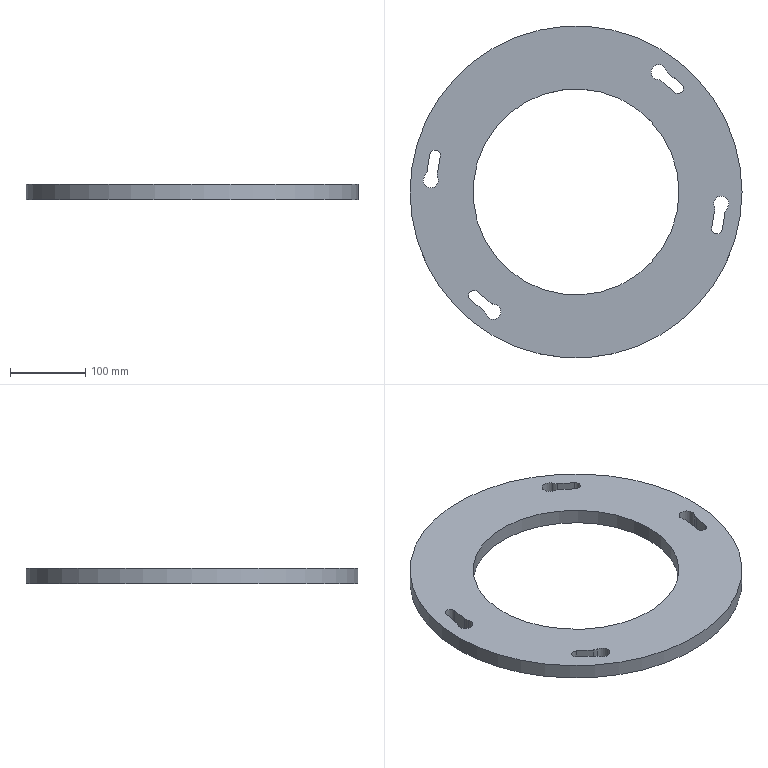Part | NX | 1 solid | 28 faces | box 440 x 440 x 20 mm | volume 1811359 mm3 | cylinder 18 | plane 10 | commonest cylinder face diameters 26 x8 14 x4 20 x4 273 x1 440 x1
STEP:
#1=CARTESIAN_POINT('',(182.981,-18.897,-20.));
#2=VERTEX_POINT('',#1);
#3=CARTESIAN_POINT('',(200.129,-21.798,-20.));
#4=VERTEX_POINT('',#3);
#5=CARTESIAN_POINT('',(192.378,-15.478,-20.));
#6=DIRECTION('',(0.,0.,-1.));
#7=DIRECTION('',(-1.,0.,0.));
#8=AXIS2_PLACEMENT_3D('',#5,#6,#7);
#9=CIRCLE('',#8,10.);
#10=EDGE_CURVE('',#2,#4,#9,.T.);
#11=ORIENTED_EDGE('',*,*,#10,.T.);
#12=CARTESIAN_POINT('',(200.129,-21.798,0.));
#13=VERTEX_POINT('',#12);
#14=CARTESIAN_POINT('',(200.129,-21.798,-20.));
#15=DIRECTION('',(0.,0.,1.));
#16=VECTOR('',#15,1000.);
#17=LINE('',#14,#16);
#18=EDGE_CURVE('',#4,#13,#17,.T.);
#19=ORIENTED_EDGE('',*,*,#18,.T.);
#20=CARTESIAN_POINT('',(182.981,-18.897,0.));
#21=VERTEX_POINT('',#20);
#22=CARTESIAN_POINT('',(192.378,-15.478,0.));
#23=DIRECTION('',(0.,0.,-1.));
#24=DIRECTION('',(-1.,0.,0.));
#25=AXIS2_PLACEMENT_3D('',#22,#23,#24);
#26=CIRCLE('',#25,10.);
#27=EDGE_CURVE('',#21,#13,#26,.T.);
#28=ORIENTED_EDGE('',*,*,#27,.F.);
#29=CARTESIAN_POINT('',(182.981,-18.897,-20.));
#30=DIRECTION('',(0.,0.,1.));
#31=VECTOR('',#30,1000.);
#32=LINE('',#29,#31);
#33=EDGE_CURVE('',#21,#2,#32,.F.);
#34=ORIENTED_EDGE('',*,*,#33,.T.);
#35=EDGE_LOOP('',(#11,#19,#28,#34));
#36=FACE_BOUND('',#35,.T.);
#37=CARTESIAN_POINT('',(192.378,-15.478,-20.));
#38=DIRECTION('',(0.,0.,1.));
#39=DIRECTION('',(1.,0.,0.));
#40=AXIS2_PLACEMENT_3D('',#37,#38,#39);
#41=CYLINDRICAL_SURFACE('',#40,10.);
#42=ADVANCED_FACE('',(#36),#41,.F.);
#43=CARTESIAN_POINT('',(197.386,-27.845,0.));
#44=VERTEX_POINT('',#43);
#45=CARTESIAN_POINT('',(193.67,-49.817,0.));
#46=VERTEX_POINT('',#45);
#47=CARTESIAN_POINT('',(198.089,-23.687,0.));
#48=DIRECTION('',(-0.1668,-0.986,0.));
#49=VECTOR('',#48,1000.);
#50=LINE('',#47,#49);
#51=EDGE_CURVE('',#44,#46,#50,.T.);
#52=ORIENTED_EDGE('',*,*,#51,.F.);
#53=CARTESIAN_POINT('',(197.386,-27.845,-20.));
#54=VERTEX_POINT('',#53);
#55=CARTESIAN_POINT('',(197.386,-27.845,-20.));
#56=DIRECTION('',(0.,0.,1.));
#57=VECTOR('',#56,1000.);
#58=LINE('',#55,#57);
#59=EDGE_CURVE('',#44,#54,#58,.F.);
#60=ORIENTED_EDGE('',*,*,#59,.T.);
#61=CARTESIAN_POINT('',(193.67,-49.817,-20.));
#62=VERTEX_POINT('',#61);
#63=CARTESIAN_POINT('',(198.089,-23.687,-20.));
#64=DIRECTION('',(-0.1668,-0.986,0.));
#65=VECTOR('',#64,1000.);
#66=LINE('',#63,#65);
#67=EDGE_CURVE('',#54,#62,#66,.T.);
#68=ORIENTED_EDGE('',*,*,#67,.T.);
#69=CARTESIAN_POINT('',(193.67,-49.817,-20.));
#70=DIRECTION('',(0.,0.,1.));
#71=VECTOR('',#70,1000.);
#72=LINE('',#69,#71);
#73=EDGE_CURVE('',#62,#46,#72,.T.);
#74=ORIENTED_EDGE('',*,*,#73,.T.);
#75=EDGE_LOOP('',(#52,#60,#68,#74));
#76=FACE_BOUND('',#75,.T.);
#77=CARTESIAN_POINT('',(198.089,-23.687,-20.));
#78=DIRECTION('',(-0.986,0.1668,0.));
#79=DIRECTION('',(-0.1668,-0.986,0.));
#80=AXIS2_PLACEMENT_3D('',#77,#78,#79);
#81=PLANE('',#80);
#82=ADVANCED_FACE('',(#76),#81,.T.);
#83=CARTESIAN_POINT('',(179.866,-47.482,0.));
#84=VERTEX_POINT('',#83);
#85=CARTESIAN_POINT('',(186.768,-48.649,0.));
#86=DIRECTION('',(0.,0.,-1.));
#87=DIRECTION('',(-1.,0.,0.));
#88=AXIS2_PLACEMENT_3D('',#85,#86,#87);
#89=CIRCLE('',#88,7.);
#90=EDGE_CURVE('',#46,#84,#89,.T.);
#91=ORIENTED_EDGE('',*,*,#90,.F.);
#92=ORIENTED_EDGE('',*,*,#73,.F.);
#93=CARTESIAN_POINT('',(179.866,-47.482,-20.));
#94=VERTEX_POINT('',#93);
#95=CARTESIAN_POINT('',(186.768,-48.649,-20.));
#96=DIRECTION('',(0.,0.,-1.));
#97=DIRECTION('',(-1.,0.,0.));
#98=AXIS2_PLACEMENT_3D('',#95,#96,#97);
#99=CIRCLE('',#98,7.);
#100=EDGE_CURVE('',#62,#94,#99,.T.);
#101=ORIENTED_EDGE('',*,*,#100,.T.);
#102=CARTESIAN_POINT('',(179.866,-47.482,-20.));
#103=DIRECTION('',(0.,0.,1.));
#104=VECTOR('',#103,1000.);
#105=LINE('',#102,#104);
#106=EDGE_CURVE('',#94,#84,#105,.T.);
#107=ORIENTED_EDGE('',*,*,#106,.T.);
#108=EDGE_LOOP('',(#91,#92,#101,#107));
#109=FACE_BOUND('',#108,.T.);
#110=CARTESIAN_POINT('',(186.768,-48.649,-20.));
#111=DIRECTION('',(0.,0.,1.));
#112=DIRECTION('',(1.,0.,0.));
#113=AXIS2_PLACEMENT_3D('',#110,#111,#112);
#114=CYLINDRICAL_SURFACE('',#113,7.);
#115=ADVANCED_FACE('',(#109),#114,.F.);
#116=CARTESIAN_POINT('',(139.978,142.815,0.));
#117=VERTEX_POINT('',#116);
#118=CARTESIAN_POINT('',(131.054,132.027,0.));
#119=VERTEX_POINT('',#118);
#120=CARTESIAN_POINT('',(135.516,137.421,0.));
#121=DIRECTION('',(0.,0.,-1.));
#122=DIRECTION('',(-1.,0.,0.));
#123=AXIS2_PLACEMENT_3D('',#120,#121,#122);
#124=CIRCLE('',#123,7.);
#125=EDGE_CURVE('',#117,#119,#124,.T.);
#126=ORIENTED_EDGE('',*,*,#125,.F.);
#127=CARTESIAN_POINT('',(139.978,142.815,-20.));
#128=VERTEX_POINT('',#127);
#129=CARTESIAN_POINT('',(139.978,142.815,-20.));
#130=DIRECTION('',(0.,0.,1.));
#131=VECTOR('',#130,1000.);
#132=LINE('',#129,#131);
#133=EDGE_CURVE('',#128,#117,#132,.T.);
#134=ORIENTED_EDGE('',*,*,#133,.F.);
#135=CARTESIAN_POINT('',(131.054,132.027,-20.));
#136=VERTEX_POINT('',#135);
#137=CARTESIAN_POINT('',(135.516,137.421,-20.));
#138=DIRECTION('',(0.,0.,-1.));
#139=DIRECTION('',(-1.,0.,0.));
#140=AXIS2_PLACEMENT_3D('',#137,#138,#139);
#141=CIRCLE('',#140,7.);
#142=EDGE_CURVE('',#128,#136,#141,.T.);
#143=ORIENTED_EDGE('',*,*,#142,.T.);
#144=CARTESIAN_POINT('',(131.054,132.027,-20.));
#145=DIRECTION('',(0.,0.,1.));
#146=VECTOR('',#145,1000.);
#147=LINE('',#144,#146);
#148=EDGE_CURVE('',#136,#119,#147,.T.);
#149=ORIENTED_EDGE('',*,*,#148,.T.);
#150=EDGE_LOOP('',(#126,#134,#143,#149));
#151=FACE_BOUND('',#150,.T.);
#152=CARTESIAN_POINT('',(135.516,137.421,-20.));
#153=DIRECTION('',(0.,0.,1.));
#154=DIRECTION('',(1.,0.,0.));
#155=AXIS2_PLACEMENT_3D('',#152,#153,#154);
#156=CYLINDRICAL_SURFACE('',#155,7.);
#157=ADVANCED_FACE('',(#151),#156,.F.);
#158=CARTESIAN_POINT('',(113.883,146.232,-20.));
#159=VERTEX_POINT('',#158);
#160=CARTESIAN_POINT('',(131.054,132.027,-20.));
#161=DIRECTION('',(-0.7705,0.6374,0.));
#162=VECTOR('',#161,1000.);
#163=LINE('',#160,#162);
#164=EDGE_CURVE('',#136,#159,#163,.T.);
#165=ORIENTED_EDGE('',*,*,#164,.T.);
#166=CARTESIAN_POINT('',(113.883,146.232,0.));
#167=VERTEX_POINT('',#166);
#168=CARTESIAN_POINT('',(113.883,146.232,-20.));
#169=DIRECTION('',(0.,0.,1.));
#170=VECTOR('',#169,1000.);
#171=LINE('',#168,#170);
#172=EDGE_CURVE('',#159,#167,#171,.T.);
#173=ORIENTED_EDGE('',*,*,#172,.T.);
#174=CARTESIAN_POINT('',(131.054,132.027,0.));
#175=DIRECTION('',(-0.7705,0.6374,0.));
#176=VECTOR('',#175,1000.);
#177=LINE('',#174,#176);
#178=EDGE_CURVE('',#119,#167,#177,.T.);
#179=ORIENTED_EDGE('',*,*,#178,.F.);
#180=ORIENTED_EDGE('',*,*,#148,.F.);
#181=EDGE_LOOP('',(#165,#173,#179,#180));
#182=FACE_BOUND('',#181,.T.);
#183=CARTESIAN_POINT('',(131.054,132.027,-20.));
#184=DIRECTION('',(0.6374,0.7705,0.));
#185=DIRECTION('',(-0.7705,0.6374,0.));
#186=AXIS2_PLACEMENT_3D('',#183,#184,#185);
#187=PLANE('',#186);
#188=ADVANCED_FACE('',(#182),#187,.T.);
#189=CARTESIAN_POINT('',(107.856,149.017,0.));
#190=VERTEX_POINT('',#189);
#191=CARTESIAN_POINT('',(118.942,162.418,0.));
#192=VERTEX_POINT('',#191);
#193=CARTESIAN_POINT('',(109.594,158.865,0.));
#194=DIRECTION('',(0.,0.,-1.));
#195=DIRECTION('',(-1.,0.,0.));
#196=AXIS2_PLACEMENT_3D('',#193,#194,#195);
#197=CIRCLE('',#196,10.);
#198=EDGE_CURVE('',#190,#192,#197,.T.);
#199=ORIENTED_EDGE('',*,*,#198,.F.);
#200=CARTESIAN_POINT('',(107.856,149.017,-20.));
#201=VERTEX_POINT('',#200);
#202=CARTESIAN_POINT('',(107.856,149.017,-20.));
#203=DIRECTION('',(0.,0.,1.));
#204=VECTOR('',#203,1000.);
#205=LINE('',#202,#204);
#206=EDGE_CURVE('',#190,#201,#205,.F.);
#207=ORIENTED_EDGE('',*,*,#206,.T.);
#208=CARTESIAN_POINT('',(118.942,162.418,-20.));
#209=VERTEX_POINT('',#208);
#210=CARTESIAN_POINT('',(109.594,158.865,-20.));
#211=DIRECTION('',(0.,0.,-1.));
#212=DIRECTION('',(-1.,0.,0.));
#213=AXIS2_PLACEMENT_3D('',#210,#211,#212);
#214=CIRCLE('',#213,10.);
#215=EDGE_CURVE('',#201,#209,#214,.T.);
#216=ORIENTED_EDGE('',*,*,#215,.T.);
#217=CARTESIAN_POINT('',(118.942,162.418,-20.));
#218=DIRECTION('',(0.,0.,1.));
#219=VECTOR('',#218,1000.);
#220=LINE('',#217,#219);
#221=EDGE_CURVE('',#209,#192,#220,.T.);
#222=ORIENTED_EDGE('',*,*,#221,.T.);
#223=EDGE_LOOP('',(#199,#207,#216,#222));
#224=FACE_BOUND('',#223,.T.);
#225=CARTESIAN_POINT('',(109.594,158.865,-20.));
#226=DIRECTION('',(0.,0.,1.));
#227=DIRECTION('',(1.,0.,0.));
#228=AXIS2_PLACEMENT_3D('',#225,#226,#227);
#229=CYLINDRICAL_SURFACE('',#228,10.);
#230=ADVANCED_FACE('',(#224),#229,.F.);
#231=CARTESIAN_POINT('',(-107.856,-149.017,-20.));
#232=VERTEX_POINT('',#231);
#233=CARTESIAN_POINT('',(-118.942,-162.418,-20.));
#234=VERTEX_POINT('',#233);
#235=CARTESIAN_POINT('',(-109.594,-158.865,-20.));
#236=DIRECTION('',(0.,0.,-1.));
#237=DIRECTION('',(1.,0.,0.));
#238=AXIS2_PLACEMENT_3D('',#235,#236,#237);
#239=CIRCLE('',#238,10.);
#240=EDGE_CURVE('',#232,#234,#239,.T.);
#241=ORIENTED_EDGE('',*,*,#240,.T.);
#242=CARTESIAN_POINT('',(-118.942,-162.418,0.));
#243=VERTEX_POINT('',#242);
#244=CARTESIAN_POINT('',(-118.942,-162.418,-20.));
#245=DIRECTION('',(0.,0.,1.));
#246=VECTOR('',#245,1000.);
#247=LINE('',#244,#246);
#248=EDGE_CURVE('',#234,#243,#247,.T.);
#249=ORIENTED_EDGE('',*,*,#248,.T.);
#250=CARTESIAN_POINT('',(-107.856,-149.017,0.));
#251=VERTEX_POINT('',#250);
#252=CARTESIAN_POINT('',(-109.594,-158.865,0.));
#253=DIRECTION('',(0.,0.,-1.));
#254=DIRECTION('',(1.,0.,0.));
#255=AXIS2_PLACEMENT_3D('',#252,#253,#254);
#256=CIRCLE('',#255,10.);
#257=EDGE_CURVE('',#251,#243,#256,.T.);
#258=ORIENTED_EDGE('',*,*,#257,.F.);
#259=CARTESIAN_POINT('',(-107.856,-149.017,-20.));
#260=DIRECTION('',(0.,0.,1.));
#261=VECTOR('',#260,1000.);
#262=LINE('',#259,#261);
#263=EDGE_CURVE('',#251,#232,#262,.F.);
#264=ORIENTED_EDGE('',*,*,#263,.T.);
#265=EDGE_LOOP('',(#241,#249,#258,#264));
#266=FACE_BOUND('',#265,.T.);
#267=CARTESIAN_POINT('',(-109.594,-158.865,-20.));
#268=DIRECTION('',(0.,0.,1.));
#269=DIRECTION('',(1.,0.,0.));
#270=AXIS2_PLACEMENT_3D('',#267,#268,#269);
#271=CYLINDRICAL_SURFACE('',#270,10.);
#272=ADVANCED_FACE('',(#266),#271,.F.);
#273=CARTESIAN_POINT('',(-122.807,-157.019,0.));
#274=VERTEX_POINT('',#273);
#275=CARTESIAN_POINT('',(-139.978,-142.815,0.));
#276=VERTEX_POINT('',#275);
#277=CARTESIAN_POINT('',(-119.558,-159.707,0.));
#278=DIRECTION('',(-0.7705,0.6374,0.));
#279=VECTOR('',#278,1000.);
#280=LINE('',#277,#279);
#281=EDGE_CURVE('',#274,#276,#280,.T.);
#282=ORIENTED_EDGE('',*,*,#281,.F.);
#283=CARTESIAN_POINT('',(-122.807,-157.019,-20.));
#284=VERTEX_POINT('',#283);
#285=CARTESIAN_POINT('',(-122.807,-157.019,-20.));
#286=DIRECTION('',(0.,0.,1.));
#287=VECTOR('',#286,1000.);
#288=LINE('',#285,#287);
#289=EDGE_CURVE('',#274,#284,#288,.F.);
#290=ORIENTED_EDGE('',*,*,#289,.T.);
#291=CARTESIAN_POINT('',(-139.978,-142.815,-20.));
#292=VERTEX_POINT('',#291);
#293=CARTESIAN_POINT('',(-119.558,-159.707,-20.));
#294=DIRECTION('',(-0.7705,0.6374,0.));
#295=VECTOR('',#294,1000.);
#296=LINE('',#293,#295);
#297=EDGE_CURVE('',#284,#292,#296,.T.);
#298=ORIENTED_EDGE('',*,*,#297,.T.);
#299=CARTESIAN_POINT('',(-139.978,-142.815,-20.));
#300=DIRECTION('',(0.,0.,1.));
#301=VECTOR('',#300,1000.);
#302=LINE('',#299,#301);
#303=EDGE_CURVE('',#292,#276,#302,.T.);
#304=ORIENTED_EDGE('',*,*,#303,.T.);
#305=EDGE_LOOP('',(#282,#290,#298,#304));
#306=FACE_BOUND('',#305,.T.);
#307=CARTESIAN_POINT('',(-119.558,-159.707,-20.));
#308=DIRECTION('',(0.6374,0.7705,0.));
#309=DIRECTION('',(-0.7705,0.6374,0.));
#310=AXIS2_PLACEMENT_3D('',#307,#308,#309);
#311=PLANE('',#310);
#312=ADVANCED_FACE('',(#306),#311,.T.);
#313=CARTESIAN_POINT('',(-131.054,-132.027,0.));
#314=VERTEX_POINT('',#313);
#315=CARTESIAN_POINT('',(-135.516,-137.421,0.));
#316=DIRECTION('',(0.,0.,-1.));
#317=DIRECTION('',(1.,0.,0.));
#318=AXIS2_PLACEMENT_3D('',#315,#316,#317);
#319=CIRCLE('',#318,7.);
#320=EDGE_CURVE('',#276,#314,#319,.T.);
#321=ORIENTED_EDGE('',*,*,#320,.F.);
#322=ORIENTED_EDGE('',*,*,#303,.F.);
#323=CARTESIAN_POINT('',(-131.054,-132.027,-20.));
#324=VERTEX_POINT('',#323);
#325=CARTESIAN_POINT('',(-135.516,-137.421,-20.));
#326=DIRECTION('',(0.,0.,-1.));
#327=DIRECTION('',(1.,0.,0.));
#328=AXIS2_PLACEMENT_3D('',#325,#326,#327);
#329=CIRCLE('',#328,7.);
#330=EDGE_CURVE('',#292,#324,#329,.T.);
#331=ORIENTED_EDGE('',*,*,#330,.T.);
#332=CARTESIAN_POINT('',(-131.054,-132.027,-20.));
#333=DIRECTION('',(0.,0.,1.));
#334=VECTOR('',#333,1000.);
#335=LINE('',#332,#334);
#336=EDGE_CURVE('',#324,#314,#335,.T.);
#337=ORIENTED_EDGE('',*,*,#336,.T.);
#338=EDGE_LOOP('',(#321,#322,#331,#337));
#339=FACE_BOUND('',#338,.T.);
#340=CARTESIAN_POINT('',(-135.516,-137.421,-20.));
#341=DIRECTION('',(0.,0.,1.));
#342=DIRECTION('',(1.,0.,0.));
#343=AXIS2_PLACEMENT_3D('',#340,#341,#342);
#344=CYLINDRICAL_SURFACE('',#343,7.);
#345=ADVANCED_FACE('',(#339),#344,.F.);
#346=CARTESIAN_POINT('',(-179.866,47.482,0.));
#347=VERTEX_POINT('',#346);
#348=CARTESIAN_POINT('',(-193.67,49.817,0.));
#349=VERTEX_POINT('',#348);
#350=CARTESIAN_POINT('',(-186.768,48.649,0.));
#351=DIRECTION('',(0.,0.,1.));
#352=DIRECTION('',(1.,0.,0.));
#353=AXIS2_PLACEMENT_3D('',#350,#351,#352);
#354=CIRCLE('',#353,7.);
#355=EDGE_CURVE('',#347,#349,#354,.T.);
#356=ORIENTED_EDGE('',*,*,#355,.T.);
#357=CARTESIAN_POINT('',(-193.67,49.817,-20.));
#358=VERTEX_POINT('',#357);
#359=CARTESIAN_POINT('',(-193.67,49.817,-20.));
#360=DIRECTION('',(0.,0.,1.));
#361=VECTOR('',#360,1000.);
#362=LINE('',#359,#361);
#363=EDGE_CURVE('',#358,#349,#362,.T.);
#364=ORIENTED_EDGE('',*,*,#363,.F.);
#365=CARTESIAN_POINT('',(-179.866,47.482,-20.));
#366=VERTEX_POINT('',#365);
#367=CARTESIAN_POINT('',(-186.768,48.649,-20.));
#368=DIRECTION('',(0.,0.,1.));
#369=DIRECTION('',(1.,0.,0.));
#370=AXIS2_PLACEMENT_3D('',#367,#368,#369);
#371=CIRCLE('',#370,7.);
#372=EDGE_CURVE('',#366,#358,#371,.T.);
#373=ORIENTED_EDGE('',*,*,#372,.F.);
#374=CARTESIAN_POINT('',(-179.866,47.482,-20.));
#375=DIRECTION('',(0.,0.,1.));
#376=VECTOR('',#375,1000.);
#377=LINE('',#374,#376);
#378=EDGE_CURVE('',#366,#347,#377,.T.);
#379=ORIENTED_EDGE('',*,*,#378,.T.);
#380=EDGE_LOOP('',(#356,#364,#373,#379));
#381=FACE_BOUND('',#380,.T.);
#382=CARTESIAN_POINT('',(-186.768,48.649,-20.));
#383=DIRECTION('',(0.,0.,1.));
#384=DIRECTION('',(1.,0.,0.));
#385=AXIS2_PLACEMENT_3D('',#382,#383,#384);
#386=CYLINDRICAL_SURFACE('',#385,7.);
#387=ADVANCED_FACE('',(#381),#386,.F.);
#388=CARTESIAN_POINT('',(-183.582,25.51,-20.));
#389=VERTEX_POINT('',#388);
#390=CARTESIAN_POINT('',(-184.285,21.352,-20.));
#391=DIRECTION('',(0.1668,0.986,0.));
#392=VECTOR('',#391,1000.);
#393=LINE('',#390,#392);
#394=EDGE_CURVE('',#389,#366,#393,.T.);
#395=ORIENTED_EDGE('',*,*,#394,.F.);
#396=CARTESIAN_POINT('',(-183.582,25.51,0.));
#397=VERTEX_POINT('',#396);
#398=CARTESIAN_POINT('',(-183.582,25.51,-20.));
#399=DIRECTION('',(0.,0.,1.));
#400=VECTOR('',#399,1000.);
#401=LINE('',#398,#400);
#402=EDGE_CURVE('',#389,#397,#401,.T.);
#403=ORIENTED_EDGE('',*,*,#402,.T.);
#404=CARTESIAN_POINT('',(-184.285,21.352,0.));
#405=DIRECTION('',(0.1668,0.986,0.));
#406=VECTOR('',#405,1000.);
#407=LINE('',#404,#406);
#408=EDGE_CURVE('',#397,#347,#407,.T.);
#409=ORIENTED_EDGE('',*,*,#408,.T.);
#410=ORIENTED_EDGE('',*,*,#378,.F.);
#411=EDGE_LOOP('',(#395,#403,#409,#410));
#412=FACE_BOUND('',#411,.T.);
#413=CARTESIAN_POINT('',(-184.285,21.352,-20.));
#414=DIRECTION('',(0.986,-0.1668,0.));
#415=DIRECTION('',(0.1668,0.986,0.));
#416=AXIS2_PLACEMENT_3D('',#413,#414,#415);
#417=PLANE('',#416);
#418=ADVANCED_FACE('',(#412),#417,.F.);
#419=CARTESIAN_POINT('',(-200.129,21.798,0.));
#420=VERTEX_POINT('',#419);
#421=CARTESIAN_POINT('',(-182.981,18.897,0.));
#422=VERTEX_POINT('',#421);
#423=CARTESIAN_POINT('',(-192.378,15.478,0.));
#424=DIRECTION('',(0.,0.,1.));
#425=DIRECTION('',(1.,0.,0.));
#426=AXIS2_PLACEMENT_3D('',#423,#424,#425);
#427=CIRCLE('',#426,10.);
#428=EDGE_CURVE('',#420,#422,#427,.T.);
#429=ORIENTED_EDGE('',*,*,#428,.T.);
#430=CARTESIAN_POINT('',(-182.981,18.897,-20.));
#431=VERTEX_POINT('',#430);
#432=CARTESIAN_POINT('',(-182.981,18.897,-20.));
#433=DIRECTION('',(0.,0.,1.));
#434=VECTOR('',#433,1000.);
#435=LINE('',#432,#434);
#436=EDGE_CURVE('',#422,#431,#435,.F.);
#437=ORIENTED_EDGE('',*,*,#436,.T.);
#438=CARTESIAN_POINT('',(-200.129,21.798,-20.));
#439=VERTEX_POINT('',#438);
#440=CARTESIAN_POINT('',(-192.378,15.478,-20.));
#441=DIRECTION('',(0.,0.,1.));
#442=DIRECTION('',(1.,0.,0.));
#443=AXIS2_PLACEMENT_3D('',#440,#441,#442);
#444=CIRCLE('',#443,10.);
#445=EDGE_CURVE('',#439,#431,#444,.T.);
#446=ORIENTED_EDGE('',*,*,#445,.F.);
#447=CARTESIAN_POINT('',(-200.129,21.798,-20.));
#448=DIRECTION('',(0.,0.,1.));
#449=VECTOR('',#448,1000.);
#450=LINE('',#447,#449);
#451=EDGE_CURVE('',#439,#420,#450,.T.);
#452=ORIENTED_EDGE('',*,*,#451,.T.);
#453=EDGE_LOOP('',(#429,#437,#446,#452));
#454=FACE_BOUND('',#453,.T.);
#455=CARTESIAN_POINT('',(-192.378,15.478,-20.));
#456=DIRECTION('',(0.,0.,1.));
#457=DIRECTION('',(1.,0.,0.));
#458=AXIS2_PLACEMENT_3D('',#455,#456,#457);
#459=CYLINDRICAL_SURFACE('',#458,10.);
#460=ADVANCED_FACE('',(#454),#459,.F.);
#461=CARTESIAN_POINT('',(122.807,157.019,0.));
#462=VERTEX_POINT('',#461);
#463=CARTESIAN_POINT('',(119.558,159.707,0.));
#464=DIRECTION('',(0.7705,-0.6374,0.));
#465=VECTOR('',#464,1000.);
#466=LINE('',#463,#465);
#467=EDGE_CURVE('',#462,#117,#466,.T.);
#468=ORIENTED_EDGE('',*,*,#467,.F.);
#469=CARTESIAN_POINT('',(122.807,157.019,-20.));
#470=VERTEX_POINT('',#469);
#471=CARTESIAN_POINT('',(122.807,157.019,-20.));
#472=DIRECTION('',(0.,0.,1.));
#473=VECTOR('',#472,1000.);
#474=LINE('',#471,#473);
#475=EDGE_CURVE('',#462,#470,#474,.F.);
#476=ORIENTED_EDGE('',*,*,#475,.T.);
#477=CARTESIAN_POINT('',(119.558,159.707,-20.));
#478=DIRECTION('',(0.7705,-0.6374,0.));
#479=VECTOR('',#478,1000.);
#480=LINE('',#477,#479);
#481=EDGE_CURVE('',#470,#128,#480,.T.);
#482=ORIENTED_EDGE('',*,*,#481,.T.);
#483=ORIENTED_EDGE('',*,*,#133,.T.);
#484=EDGE_LOOP('',(#468,#476,#482,#483));
#485=FACE_BOUND('',#484,.T.);
#486=CARTESIAN_POINT('',(119.558,159.707,-20.));
#487=DIRECTION('',(-0.6374,-0.7705,0.));
#488=DIRECTION('',(0.7705,-0.6374,0.));
#489=AXIS2_PLACEMENT_3D('',#486,#487,#488);
#490=PLANE('',#489);
#491=ADVANCED_FACE('',(#485),#490,.T.);
#492=CARTESIAN_POINT('',(-113.883,-146.232,-20.));
#493=VERTEX_POINT('',#492);
#494=CARTESIAN_POINT('',(-131.054,-132.027,-20.));
#495=DIRECTION('',(0.7705,-0.6374,0.));
#496=VECTOR('',#495,1000.);
#497=LINE('',#494,#496);
#498=EDGE_CURVE('',#324,#493,#497,.T.);
#499=ORIENTED_EDGE('',*,*,#498,.T.);
#500=CARTESIAN_POINT('',(-113.883,-146.232,0.));
#501=VERTEX_POINT('',#500);
#502=CARTESIAN_POINT('',(-113.883,-146.232,-20.));
#503=DIRECTION('',(0.,0.,1.));
#504=VECTOR('',#503,1000.);
#505=LINE('',#502,#504);
#506=EDGE_CURVE('',#493,#501,#505,.T.);
#507=ORIENTED_EDGE('',*,*,#506,.T.);
#508=CARTESIAN_POINT('',(-131.054,-132.027,0.));
#509=DIRECTION('',(0.7705,-0.6374,0.));
#510=VECTOR('',#509,1000.);
#511=LINE('',#508,#510);
#512=EDGE_CURVE('',#314,#501,#511,.T.);
#513=ORIENTED_EDGE('',*,*,#512,.F.);
#514=ORIENTED_EDGE('',*,*,#336,.F.);
#515=EDGE_LOOP('',(#499,#507,#513,#514));
#516=FACE_BOUND('',#515,.T.);
#517=CARTESIAN_POINT('',(-131.054,-132.027,-20.));
#518=DIRECTION('',(-0.6374,-0.7705,0.));
#519=DIRECTION('',(0.7705,-0.6374,0.));
#520=AXIS2_PLACEMENT_3D('',#517,#518,#519);
#521=PLANE('',#520);
#522=ADVANCED_FACE('',(#516),#521,.T.);
#523=CARTESIAN_POINT('',(136.5,0.,-20.));
#524=VERTEX_POINT('',#523);
#525=CARTESIAN_POINT('',(0.,0.,-20.));
#526=DIRECTION('',(0.,0.,1.));
#527=DIRECTION('',(1.,0.,0.));
#528=AXIS2_PLACEMENT_3D('',#525,#526,#527);
#529=CIRCLE('',#528,136.5);
#530=EDGE_CURVE('',#524,#524,#529,.T.);
#531=ORIENTED_EDGE('',*,*,#530,.F.);
#532=EDGE_LOOP('',(#531));
#533=FACE_BOUND('',#532,.T.);
#534=CARTESIAN_POINT('',(136.5,0.,0.));
#535=VERTEX_POINT('',#534);
#536=CARTESIAN_POINT('',(0.,0.,0.));
#537=DIRECTION('',(0.,0.,1.));
#538=DIRECTION('',(1.,0.,0.));
#539=AXIS2_PLACEMENT_3D('',#536,#537,#538);
#540=CIRCLE('',#539,136.5);
#541=EDGE_CURVE('',#535,#535,#540,.T.);
#542=ORIENTED_EDGE('',*,*,#541,.T.);
#543=EDGE_LOOP('',(#542));
#544=FACE_BOUND('',#543,.T.);
#545=CARTESIAN_POINT('',(0.,0.,-20.));
#546=DIRECTION('',(0.,0.,1.));
#547=DIRECTION('',(1.,0.,0.));
#548=AXIS2_PLACEMENT_3D('',#545,#546,#547);
#549=CYLINDRICAL_SURFACE('',#548,136.5);
#550=ADVANCED_FACE('',(#533,#544),#549,.F.);
#551=CARTESIAN_POINT('',(-197.386,27.845,0.));
#552=VERTEX_POINT('',#551);
#553=CARTESIAN_POINT('',(-193.67,49.817,0.));
#554=DIRECTION('',(-0.1668,-0.986,0.));
#555=VECTOR('',#554,1000.);
#556=LINE('',#553,#555);
#557=EDGE_CURVE('',#349,#552,#556,.T.);
#558=ORIENTED_EDGE('',*,*,#557,.T.);
#559=CARTESIAN_POINT('',(-197.386,27.845,-20.));
#560=VERTEX_POINT('',#559);
#561=CARTESIAN_POINT('',(-197.386,27.845,-20.));
#562=DIRECTION('',(0.,0.,1.));
#563=VECTOR('',#562,1000.);
#564=LINE('',#561,#563);
#565=EDGE_CURVE('',#552,#560,#564,.F.);
#566=ORIENTED_EDGE('',*,*,#565,.T.);
#567=CARTESIAN_POINT('',(-193.67,49.817,-20.));
#568=DIRECTION('',(-0.1668,-0.986,0.));
#569=VECTOR('',#568,1000.);
#570=LINE('',#567,#569);
#571=EDGE_CURVE('',#358,#560,#570,.T.);
#572=ORIENTED_EDGE('',*,*,#571,.F.);
#573=ORIENTED_EDGE('',*,*,#363,.T.);
#574=EDGE_LOOP('',(#558,#566,#572,#573));
#575=FACE_BOUND('',#574,.T.);
#576=CARTESIAN_POINT('',(-193.67,49.817,-20.));
#577=DIRECTION('',(-0.986,0.1668,0.));
#578=DIRECTION('',(-0.1668,-0.986,0.));
#579=AXIS2_PLACEMENT_3D('',#576,#577,#578);
#580=PLANE('',#579);
#581=ADVANCED_FACE('',(#575),#580,.F.);
#582=CARTESIAN_POINT('',(220.,0.,-20.));
#583=VERTEX_POINT('',#582);
#584=CARTESIAN_POINT('',(0.,0.,-20.));
#585=DIRECTION('',(0.,0.,1.));
#586=DIRECTION('',(1.,0.,0.));
#587=AXIS2_PLACEMENT_3D('',#584,#585,#586);
#588=CIRCLE('',#587,220.);
#589=EDGE_CURVE('',#583,#583,#588,.T.);
#590=ORIENTED_EDGE('',*,*,#589,.T.);
#591=EDGE_LOOP('',(#590));
#592=FACE_BOUND('',#591,.T.);
#593=CARTESIAN_POINT('',(220.,0.,0.));
#594=VERTEX_POINT('',#593);
#595=CARTESIAN_POINT('',(0.,0.,0.));
#596=DIRECTION('',(0.,0.,1.));
#597=DIRECTION('',(1.,0.,0.));
#598=AXIS2_PLACEMENT_3D('',#595,#596,#597);
#599=CIRCLE('',#598,220.);
#600=EDGE_CURVE('',#594,#594,#599,.T.);
#601=ORIENTED_EDGE('',*,*,#600,.F.);
#602=EDGE_LOOP('',(#601));
#603=FACE_BOUND('',#602,.T.);
#604=CARTESIAN_POINT('',(0.,0.,-20.));
#605=DIRECTION('',(0.,0.,1.));
#606=DIRECTION('',(1.,0.,0.));
#607=AXIS2_PLACEMENT_3D('',#604,#605,#606);
#608=CYLINDRICAL_SURFACE('',#607,220.);
#609=ADVANCED_FACE('',(#592,#603),#608,.T.);
#610=CARTESIAN_POINT('',(183.582,-25.51,-20.));
#611=VERTEX_POINT('',#610);
#612=CARTESIAN_POINT('',(179.866,-47.482,-20.));
#613=DIRECTION('',(0.1668,0.986,0.));
#614=VECTOR('',#613,1000.);
#615=LINE('',#612,#614);
#616=EDGE_CURVE('',#94,#611,#615,.T.);
#617=ORIENTED_EDGE('',*,*,#616,.T.);
#618=CARTESIAN_POINT('',(183.582,-25.51,0.));
#619=VERTEX_POINT('',#618);
#620=CARTESIAN_POINT('',(183.582,-25.51,-20.));
#621=DIRECTION('',(0.,0.,1.));
#622=VECTOR('',#621,1000.);
#623=LINE('',#620,#622);
#624=EDGE_CURVE('',#611,#619,#623,.T.);
#625=ORIENTED_EDGE('',*,*,#624,.T.);
#626=CARTESIAN_POINT('',(179.866,-47.482,0.));
#627=DIRECTION('',(0.1668,0.986,0.));
#628=VECTOR('',#627,1000.);
#629=LINE('',#626,#628);
#630=EDGE_CURVE('',#84,#619,#629,.T.);
#631=ORIENTED_EDGE('',*,*,#630,.F.);
#632=ORIENTED_EDGE('',*,*,#106,.F.);
#633=EDGE_LOOP('',(#617,#625,#631,#632));
#634=FACE_BOUND('',#633,.T.);
#635=CARTESIAN_POINT('',(179.866,-47.482,-20.));
#636=DIRECTION('',(0.986,-0.1668,0.));
#637=DIRECTION('',(0.1668,0.986,0.));
#638=AXIS2_PLACEMENT_3D('',#635,#636,#637);
#639=PLANE('',#638);
#640=ADVANCED_FACE('',(#634),#639,.T.);
#641=ORIENTED_EDGE('',*,*,#589,.F.);
#642=EDGE_LOOP('',(#641));
#643=FACE_BOUND('',#642,.T.);
#644=ORIENTED_EDGE('',*,*,#445,.T.);
#645=CARTESIAN_POINT('',(-170.764,23.342,-20.));
#646=DIRECTION('',(0.,0.,1.));
#647=DIRECTION('',(1.,0.,0.));
#648=AXIS2_PLACEMENT_3D('',#645,#646,#647);
#649=CIRCLE('',#648,13.);
#650=EDGE_CURVE('',#431,#389,#649,.F.);
#651=ORIENTED_EDGE('',*,*,#650,.T.);
#652=ORIENTED_EDGE('',*,*,#394,.T.);
#653=ORIENTED_EDGE('',*,*,#372,.T.);
#654=ORIENTED_EDGE('',*,*,#571,.T.);
#655=CARTESIAN_POINT('',(-210.204,30.013,-20.));
#656=DIRECTION('',(0.,0.,1.));
#657=DIRECTION('',(1.,0.,0.));
#658=AXIS2_PLACEMENT_3D('',#655,#656,#657);
#659=CIRCLE('',#658,13.);
#660=EDGE_CURVE('',#560,#439,#659,.F.);
#661=ORIENTED_EDGE('',*,*,#660,.T.);
#662=EDGE_LOOP('',(#644,#651,#652,#653,#654,#661));
#663=FACE_BOUND('',#662,.T.);
#664=ORIENTED_EDGE('',*,*,#530,.T.);
#665=EDGE_LOOP('',(#664));
#666=FACE_BOUND('',#665,.T.);
#667=ORIENTED_EDGE('',*,*,#297,.F.);
#668=CARTESIAN_POINT('',(-131.094,-167.036,-20.));
#669=DIRECTION('',(0.,0.,1.));
#670=DIRECTION('',(1.,0.,0.));
#671=AXIS2_PLACEMENT_3D('',#668,#669,#670);
#672=CIRCLE('',#671,13.);
#673=EDGE_CURVE('',#284,#234,#672,.F.);
#674=ORIENTED_EDGE('',*,*,#673,.T.);
#675=ORIENTED_EDGE('',*,*,#240,.F.);
#676=CARTESIAN_POINT('',(-105.597,-136.215,-20.));
#677=DIRECTION('',(0.,0.,1.));
#678=DIRECTION('',(1.,0.,0.));
#679=AXIS2_PLACEMENT_3D('',#676,#677,#678);
#680=CIRCLE('',#679,13.);
#681=EDGE_CURVE('',#232,#493,#680,.F.);
#682=ORIENTED_EDGE('',*,*,#681,.T.);
#683=ORIENTED_EDGE('',*,*,#498,.F.);
#684=ORIENTED_EDGE('',*,*,#330,.F.);
#685=EDGE_LOOP('',(#667,#674,#675,#682,#683,#684));
#686=FACE_BOUND('',#685,.T.);
#687=ORIENTED_EDGE('',*,*,#215,.F.);
#688=CARTESIAN_POINT('',(105.597,136.215,-20.));
#689=DIRECTION('',(0.,0.,1.));
#690=DIRECTION('',(1.,0.,0.));
#691=AXIS2_PLACEMENT_3D('',#688,#689,#690);
#692=CIRCLE('',#691,13.);
#693=EDGE_CURVE('',#201,#159,#692,.F.);
#694=ORIENTED_EDGE('',*,*,#693,.T.);
#695=ORIENTED_EDGE('',*,*,#164,.F.);
#696=ORIENTED_EDGE('',*,*,#142,.F.);
#697=ORIENTED_EDGE('',*,*,#481,.F.);
#698=CARTESIAN_POINT('',(131.094,167.036,-20.));
#699=DIRECTION('',(0.,0.,1.));
#700=DIRECTION('',(1.,0.,0.));
#701=AXIS2_PLACEMENT_3D('',#698,#699,#700);
#702=CIRCLE('',#701,13.);
#703=EDGE_CURVE('',#470,#209,#702,.F.);
#704=ORIENTED_EDGE('',*,*,#703,.T.);
#705=EDGE_LOOP('',(#687,#694,#695,#696,#697,#704));
#706=FACE_BOUND('',#705,.T.);
#707=ORIENTED_EDGE('',*,*,#67,.F.);
#708=CARTESIAN_POINT('',(210.204,-30.013,-20.));
#709=DIRECTION('',(0.,0.,1.));
#710=DIRECTION('',(1.,0.,0.));
#711=AXIS2_PLACEMENT_3D('',#708,#709,#710);
#712=CIRCLE('',#711,13.);
#713=EDGE_CURVE('',#54,#4,#712,.F.);
#714=ORIENTED_EDGE('',*,*,#713,.T.);
#715=ORIENTED_EDGE('',*,*,#10,.F.);
#716=CARTESIAN_POINT('',(170.764,-23.342,-20.));
#717=DIRECTION('',(0.,0.,1.));
#718=DIRECTION('',(1.,0.,0.));
#719=AXIS2_PLACEMENT_3D('',#716,#717,#718);
#720=CIRCLE('',#719,13.);
#721=EDGE_CURVE('',#2,#611,#720,.F.);
#722=ORIENTED_EDGE('',*,*,#721,.T.);
#723=ORIENTED_EDGE('',*,*,#616,.F.);
#724=ORIENTED_EDGE('',*,*,#100,.F.);
#725=EDGE_LOOP('',(#707,#714,#715,#722,#723,#724));
#726=FACE_BOUND('',#725,.T.);
#727=CARTESIAN_POINT('',(0.,0.,-20.));
#728=DIRECTION('',(0.,0.,1.));
#729=DIRECTION('',(1.,0.,0.));
#730=AXIS2_PLACEMENT_3D('',#727,#728,#729);
#731=PLANE('',#730);
#732=ADVANCED_FACE('',(#643,#663,#666,#686,#706,#726),#731,.F.);
#733=ORIENTED_EDGE('',*,*,#600,.T.);
#734=EDGE_LOOP('',(#733));
#735=FACE_BOUND('',#734,.T.);
#736=ORIENTED_EDGE('',*,*,#408,.F.);
#737=CARTESIAN_POINT('',(-170.764,23.342,0.));
#738=DIRECTION('',(0.,0.,1.));
#739=DIRECTION('',(1.,0.,0.));
#740=AXIS2_PLACEMENT_3D('',#737,#738,#739);
#741=CIRCLE('',#740,13.);
#742=EDGE_CURVE('',#397,#422,#741,.T.);
#743=ORIENTED_EDGE('',*,*,#742,.T.);
#744=ORIENTED_EDGE('',*,*,#428,.F.);
#745=CARTESIAN_POINT('',(-210.204,30.013,0.));
#746=DIRECTION('',(0.,0.,1.));
#747=DIRECTION('',(1.,0.,0.));
#748=AXIS2_PLACEMENT_3D('',#745,#746,#747);
#749=CIRCLE('',#748,13.);
#750=EDGE_CURVE('',#420,#552,#749,.T.);
#751=ORIENTED_EDGE('',*,*,#750,.T.);
#752=ORIENTED_EDGE('',*,*,#557,.F.);
#753=ORIENTED_EDGE('',*,*,#355,.F.);
#754=EDGE_LOOP('',(#736,#743,#744,#751,#752,#753));
#755=FACE_BOUND('',#754,.T.);
#756=ORIENTED_EDGE('',*,*,#541,.F.);
#757=EDGE_LOOP('',(#756));
#758=FACE_BOUND('',#757,.T.);
#759=ORIENTED_EDGE('',*,*,#257,.T.);
#760=CARTESIAN_POINT('',(-131.094,-167.036,0.));
#761=DIRECTION('',(0.,0.,1.));
#762=DIRECTION('',(1.,0.,0.));
#763=AXIS2_PLACEMENT_3D('',#760,#761,#762);
#764=CIRCLE('',#763,13.);
#765=EDGE_CURVE('',#243,#274,#764,.T.);
#766=ORIENTED_EDGE('',*,*,#765,.T.);
#767=ORIENTED_EDGE('',*,*,#281,.T.);
#768=ORIENTED_EDGE('',*,*,#320,.T.);
#769=ORIENTED_EDGE('',*,*,#512,.T.);
#770=CARTESIAN_POINT('',(-105.597,-136.215,0.));
#771=DIRECTION('',(0.,0.,1.));
#772=DIRECTION('',(1.,0.,0.));
#773=AXIS2_PLACEMENT_3D('',#770,#771,#772);
#774=CIRCLE('',#773,13.);
#775=EDGE_CURVE('',#501,#251,#774,.T.);
#776=ORIENTED_EDGE('',*,*,#775,.T.);
#777=EDGE_LOOP('',(#759,#766,#767,#768,#769,#776));
#778=FACE_BOUND('',#777,.T.);
#779=ORIENTED_EDGE('',*,*,#178,.T.);
#780=CARTESIAN_POINT('',(105.597,136.215,0.));
#781=DIRECTION('',(0.,0.,1.));
#782=DIRECTION('',(1.,0.,0.));
#783=AXIS2_PLACEMENT_3D('',#780,#781,#782);
#784=CIRCLE('',#783,13.);
#785=EDGE_CURVE('',#167,#190,#784,.T.);
#786=ORIENTED_EDGE('',*,*,#785,.T.);
#787=ORIENTED_EDGE('',*,*,#198,.T.);
#788=CARTESIAN_POINT('',(131.094,167.036,0.));
#789=DIRECTION('',(0.,0.,1.));
#790=DIRECTION('',(1.,0.,0.));
#791=AXIS2_PLACEMENT_3D('',#788,#789,#790);
#792=CIRCLE('',#791,13.);
#793=EDGE_CURVE('',#192,#462,#792,.T.);
#794=ORIENTED_EDGE('',*,*,#793,.T.);
#795=ORIENTED_EDGE('',*,*,#467,.T.);
#796=ORIENTED_EDGE('',*,*,#125,.T.);
#797=EDGE_LOOP('',(#779,#786,#787,#794,#795,#796));
#798=FACE_BOUND('',#797,.T.);
#799=ORIENTED_EDGE('',*,*,#27,.T.);
#800=CARTESIAN_POINT('',(210.204,-30.013,0.));
#801=DIRECTION('',(0.,0.,1.));
#802=DIRECTION('',(1.,0.,0.));
#803=AXIS2_PLACEMENT_3D('',#800,#801,#802);
#804=CIRCLE('',#803,13.);
#805=EDGE_CURVE('',#13,#44,#804,.T.);
#806=ORIENTED_EDGE('',*,*,#805,.T.);
#807=ORIENTED_EDGE('',*,*,#51,.T.);
#808=ORIENTED_EDGE('',*,*,#90,.T.);
#809=ORIENTED_EDGE('',*,*,#630,.T.);
#810=CARTESIAN_POINT('',(170.764,-23.342,0.));
#811=DIRECTION('',(0.,0.,1.));
#812=DIRECTION('',(1.,0.,0.));
#813=AXIS2_PLACEMENT_3D('',#810,#811,#812);
#814=CIRCLE('',#813,13.);
#815=EDGE_CURVE('',#619,#21,#814,.T.);
#816=ORIENTED_EDGE('',*,*,#815,.T.);
#817=EDGE_LOOP('',(#799,#806,#807,#808,#809,#816));
#818=FACE_BOUND('',#817,.T.);
#819=CARTESIAN_POINT('',(0.,0.,0.));
#820=DIRECTION('',(0.,0.,1.));
#821=DIRECTION('',(1.,0.,0.));
#822=AXIS2_PLACEMENT_3D('',#819,#820,#821);
#823=PLANE('',#822);
#824=ADVANCED_FACE('',(#735,#755,#758,#778,#798,#818),#823,.T.);
#825=ORIENTED_EDGE('',*,*,#693,.F.);
#826=ORIENTED_EDGE('',*,*,#206,.F.);
#827=ORIENTED_EDGE('',*,*,#785,.F.);
#828=ORIENTED_EDGE('',*,*,#172,.F.);
#829=EDGE_LOOP('',(#825,#826,#827,#828));
#830=FACE_BOUND('',#829,.T.);
#831=CARTESIAN_POINT('',(105.597,136.215,-20.));
#832=DIRECTION('',(0.,0.,1.));
#833=DIRECTION('',(1.,0.,0.));
#834=AXIS2_PLACEMENT_3D('',#831,#832,#833);
#835=CYLINDRICAL_SURFACE('',#834,13.);
#836=ADVANCED_FACE('',(#830),#835,.T.);
#837=ORIENTED_EDGE('',*,*,#703,.F.);
#838=ORIENTED_EDGE('',*,*,#475,.F.);
#839=ORIENTED_EDGE('',*,*,#793,.F.);
#840=ORIENTED_EDGE('',*,*,#221,.F.);
#841=EDGE_LOOP('',(#837,#838,#839,#840));
#842=FACE_BOUND('',#841,.T.);
#843=CARTESIAN_POINT('',(131.094,167.036,-20.));
#844=DIRECTION('',(0.,0.,1.));
#845=DIRECTION('',(1.,0.,0.));
#846=AXIS2_PLACEMENT_3D('',#843,#844,#845);
#847=CYLINDRICAL_SURFACE('',#846,13.);
#848=ADVANCED_FACE('',(#842),#847,.T.);
#849=ORIENTED_EDGE('',*,*,#713,.F.);
#850=ORIENTED_EDGE('',*,*,#59,.F.);
#851=ORIENTED_EDGE('',*,*,#805,.F.);
#852=ORIENTED_EDGE('',*,*,#18,.F.);
#853=EDGE_LOOP('',(#849,#850,#851,#852));
#854=FACE_BOUND('',#853,.T.);
#855=CARTESIAN_POINT('',(210.204,-30.013,-20.));
#856=DIRECTION('',(0.,0.,1.));
#857=DIRECTION('',(1.,0.,0.));
#858=AXIS2_PLACEMENT_3D('',#855,#856,#857);
#859=CYLINDRICAL_SURFACE('',#858,13.);
#860=ADVANCED_FACE('',(#854),#859,.T.);
#861=ORIENTED_EDGE('',*,*,#721,.F.);
#862=ORIENTED_EDGE('',*,*,#33,.F.);
#863=ORIENTED_EDGE('',*,*,#815,.F.);
#864=ORIENTED_EDGE('',*,*,#624,.F.);
#865=EDGE_LOOP('',(#861,#862,#863,#864));
#866=FACE_BOUND('',#865,.T.);
#867=CARTESIAN_POINT('',(170.764,-23.342,-20.));
#868=DIRECTION('',(0.,0.,1.));
#869=DIRECTION('',(1.,0.,0.));
#870=AXIS2_PLACEMENT_3D('',#867,#868,#869);
#871=CYLINDRICAL_SURFACE('',#870,13.);
#872=ADVANCED_FACE('',(#866),#871,.T.);
#873=ORIENTED_EDGE('',*,*,#673,.F.);
#874=ORIENTED_EDGE('',*,*,#289,.F.);
#875=ORIENTED_EDGE('',*,*,#765,.F.);
#876=ORIENTED_EDGE('',*,*,#248,.F.);
#877=EDGE_LOOP('',(#873,#874,#875,#876));
#878=FACE_BOUND('',#877,.T.);
#879=CARTESIAN_POINT('',(-131.094,-167.036,-20.));
#880=DIRECTION('',(0.,0.,1.));
#881=DIRECTION('',(1.,0.,0.));
#882=AXIS2_PLACEMENT_3D('',#879,#880,#881);
#883=CYLINDRICAL_SURFACE('',#882,13.);
#884=ADVANCED_FACE('',(#878),#883,.T.);
#885=ORIENTED_EDGE('',*,*,#681,.F.);
#886=ORIENTED_EDGE('',*,*,#263,.F.);
#887=ORIENTED_EDGE('',*,*,#775,.F.);
#888=ORIENTED_EDGE('',*,*,#506,.F.);
#889=EDGE_LOOP('',(#885,#886,#887,#888));
#890=FACE_BOUND('',#889,.T.);
#891=CARTESIAN_POINT('',(-105.597,-136.215,-20.));
#892=DIRECTION('',(0.,0.,1.));
#893=DIRECTION('',(1.,0.,0.));
#894=AXIS2_PLACEMENT_3D('',#891,#892,#893);
#895=CYLINDRICAL_SURFACE('',#894,13.);
#896=ADVANCED_FACE('',(#890),#895,.T.);
#897=ORIENTED_EDGE('',*,*,#650,.F.);
#898=ORIENTED_EDGE('',*,*,#436,.F.);
#899=ORIENTED_EDGE('',*,*,#742,.F.);
#900=ORIENTED_EDGE('',*,*,#402,.F.);
#901=EDGE_LOOP('',(#897,#898,#899,#900));
#902=FACE_BOUND('',#901,.T.);
#903=CARTESIAN_POINT('',(-170.764,23.342,-20.));
#904=DIRECTION('',(0.,0.,1.));
#905=DIRECTION('',(1.,0.,0.));
#906=AXIS2_PLACEMENT_3D('',#903,#904,#905);
#907=CYLINDRICAL_SURFACE('',#906,13.);
#908=ADVANCED_FACE('',(#902),#907,.T.);
#909=ORIENTED_EDGE('',*,*,#660,.F.);
#910=ORIENTED_EDGE('',*,*,#565,.F.);
#911=ORIENTED_EDGE('',*,*,#750,.F.);
#912=ORIENTED_EDGE('',*,*,#451,.F.);
#913=EDGE_LOOP('',(#909,#910,#911,#912));
#914=FACE_BOUND('',#913,.T.);
#915=CARTESIAN_POINT('',(-210.204,30.013,-20.));
#916=DIRECTION('',(0.,0.,1.));
#917=DIRECTION('',(1.,0.,0.));
#918=AXIS2_PLACEMENT_3D('',#915,#916,#917);
#919=CYLINDRICAL_SURFACE('',#918,13.);
#920=ADVANCED_FACE('',(#914),#919,.T.);
#921=CLOSED_SHELL('',(#42,#82,#115,#157,#188,#230,#272,#312,#345,#387,#418,#460,#491,#522,#550,#581,#609,#640,#732,#824,#836,#848,#860,#872,#884,#896,#908,#920));
#922=MANIFOLD_SOLID_BREP('',#921);
#923=(LENGTH_UNIT()NAMED_UNIT(*)SI_UNIT(.MILLI.,.METRE.));
#924=UNCERTAINTY_MEASURE_WITH_UNIT(LENGTH_MEASURE(0.00001),#923,'','');
#925=(NAMED_UNIT(*)PLANE_ANGLE_UNIT()SI_UNIT($,.RADIAN.));
#926=(NAMED_UNIT(*)SI_UNIT($,.STERADIAN.)SOLID_ANGLE_UNIT());
#927=(GEOMETRIC_REPRESENTATION_CONTEXT(3)GLOBAL_UNCERTAINTY_ASSIGNED_CONTEXT((#924))GLOBAL_UNIT_ASSIGNED_CONTEXT((#923,#925,#926))REPRESENTATION_CONTEXT('',''));
#928=ADVANCED_BREP_SHAPE_REPRESENTATION('',(#922),#927);